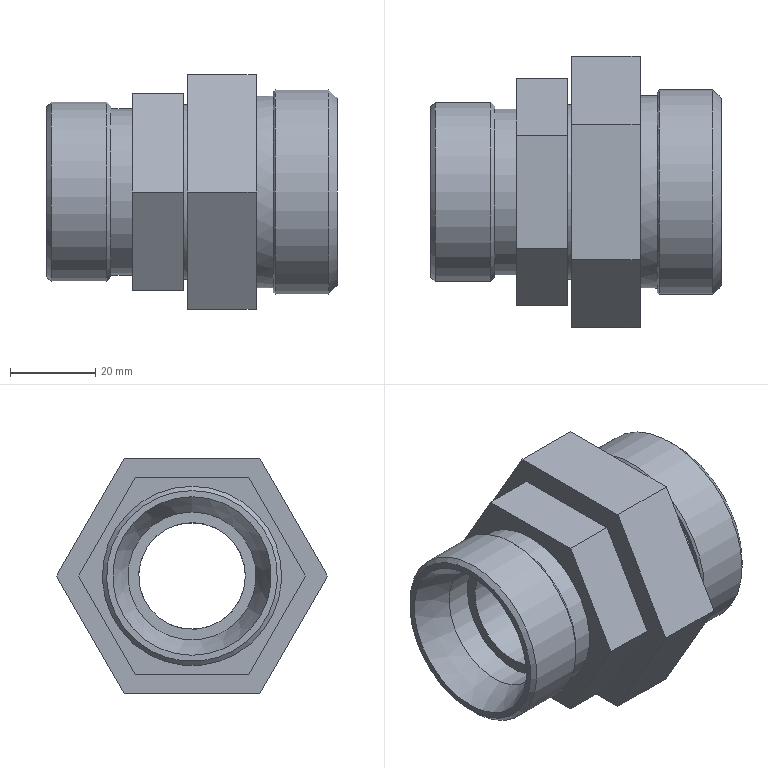Part | STEP file | HL4GZ-1.581.031 (return filter fitting weldment) | 2 solids | 41 faces | box 68 x 63.509 x 55 mm | volume 80125 mm3 | plane 23 | cylinder 9 | cone 9 | commonest cylinder face diameters 30 x3 25 x1 39 x1 41 x1 42 x1 45 x1